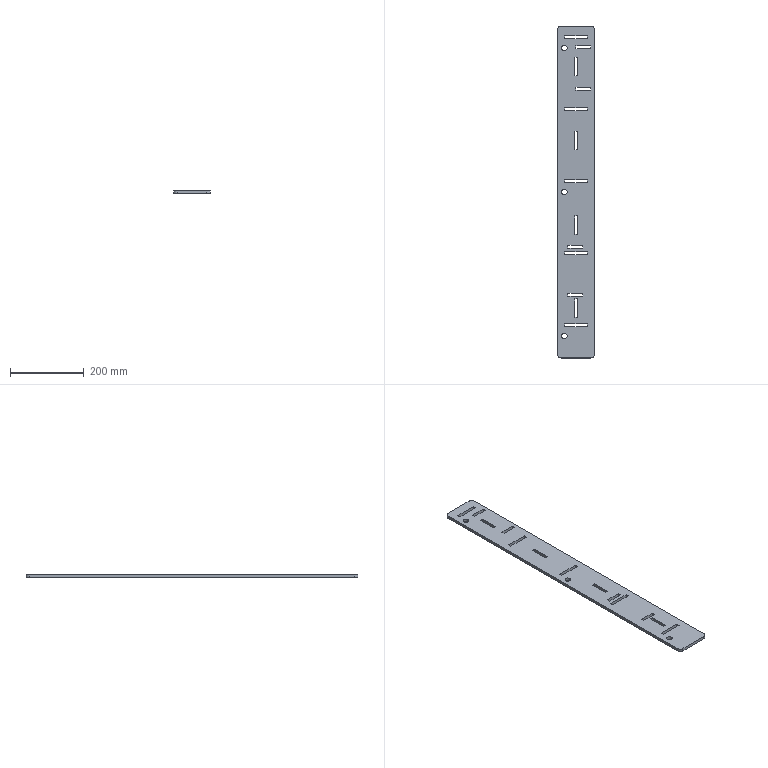Part | SolidWorks | features FlatPattern 1, SMBaseFlange 1, SheetMetal 1 | 1 solid | 68 faces | box 100 x 900 x 8 mm | volume 672832 mm3 | plane 58 | cylinder 10 | commonest cylinder face diameters 15 x6 20 x4